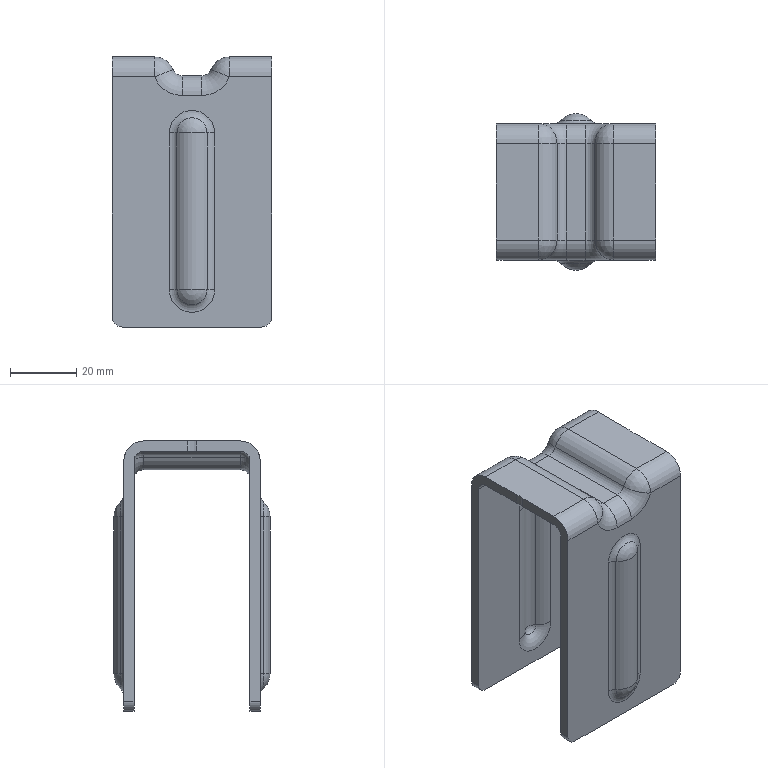Part | STEP file | PARTBODY_id310_x_t | 1 solid | 87 faces | box 48 x 47.1 x 81.415 mm | volume 29206 mm3 | cylinder 38 | sphere 17 | plane 16 | torus 16 | commonest cylinder face diameters 5.85 x10 12 x10 6.15 x6 12.3 x6 6 x4 9.576 x2